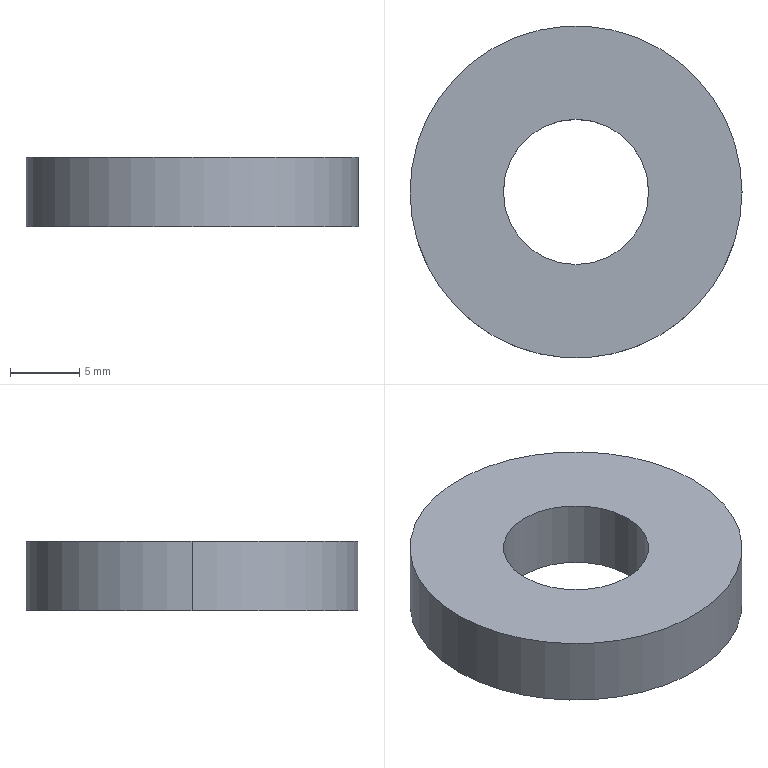Part | SolidWorks | features Extrusion 1 | 1 solid | 6 faces | box 24 x 24 x 5 mm | volume 1829 mm3 | cylinder 4 | plane 2 | commonest cylinder face diameters 10.5 x2 24 x2
STEP:
#1=CARTESIAN_POINT('',(-5.25,0.,5.));
#2=VERTEX_POINT('',#1);
#3=CARTESIAN_POINT('',(5.25,0.,5.));
#4=VERTEX_POINT('',#3);
#5=CARTESIAN_POINT('',(0.,0.,5.));
#6=DIRECTION('',(0.,0.,1.));
#7=DIRECTION('',(1.,0.,0.));
#8=AXIS2_PLACEMENT_3D('',#5,#6,#7);
#9=CIRCLE('',#8,5.25);
#10=EDGE_CURVE('',#2,#4,#9,.T.);
#11=ORIENTED_EDGE('',*,*,#10,.T.);
#12=CARTESIAN_POINT('',(5.25,0.,0.));
#13=VERTEX_POINT('',#12);
#14=CARTESIAN_POINT('',(5.25,0.,5.));
#15=DIRECTION('',(0.,0.,-1.));
#16=VECTOR('',#15,1000.);
#17=LINE('',#14,#16);
#18=EDGE_CURVE('',#4,#13,#17,.T.);
#19=ORIENTED_EDGE('',*,*,#18,.T.);
#20=CARTESIAN_POINT('',(-5.25,0.,0.));
#21=VERTEX_POINT('',#20);
#22=CARTESIAN_POINT('',(0.,0.,0.));
#23=DIRECTION('',(0.,0.,1.));
#24=DIRECTION('',(1.,0.,0.));
#25=AXIS2_PLACEMENT_3D('',#22,#23,#24);
#26=CIRCLE('',#25,5.25);
#27=EDGE_CURVE('',#21,#13,#26,.T.);
#28=ORIENTED_EDGE('',*,*,#27,.F.);
#29=CARTESIAN_POINT('',(-5.25,0.,5.));
#30=DIRECTION('',(0.,0.,-1.));
#31=VECTOR('',#30,1000.);
#32=LINE('',#29,#31);
#33=EDGE_CURVE('',#2,#21,#32,.T.);
#34=ORIENTED_EDGE('',*,*,#33,.F.);
#35=EDGE_LOOP('',(#11,#19,#28,#34));
#36=FACE_OUTER_BOUND('',#35,.T.);
#37=CARTESIAN_POINT('',(0.,0.,5.));
#38=DIRECTION('',(0.,0.,-1.));
#39=DIRECTION('',(-1.,0.,0.));
#40=AXIS2_PLACEMENT_3D('',#37,#38,#39);
#41=CYLINDRICAL_SURFACE('',#40,5.25);
#42=ADVANCED_FACE('',(#36),#41,.F.);
#43=CARTESIAN_POINT('',(12.,0.,5.));
#44=VERTEX_POINT('',#43);
#45=CARTESIAN_POINT('',(-12.,0.,5.));
#46=VERTEX_POINT('',#45);
#47=CARTESIAN_POINT('',(0.,0.,5.));
#48=DIRECTION('',(0.,0.,1.));
#49=DIRECTION('',(1.,0.,0.));
#50=AXIS2_PLACEMENT_3D('',#47,#48,#49);
#51=CIRCLE('',#50,12.);
#52=EDGE_CURVE('',#44,#46,#51,.T.);
#53=ORIENTED_EDGE('',*,*,#52,.F.);
#54=CARTESIAN_POINT('',(12.,0.,0.));
#55=VERTEX_POINT('',#54);
#56=CARTESIAN_POINT('',(12.,0.,5.));
#57=DIRECTION('',(0.,0.,-1.));
#58=VECTOR('',#57,1000.);
#59=LINE('',#56,#58);
#60=EDGE_CURVE('',#44,#55,#59,.T.);
#61=ORIENTED_EDGE('',*,*,#60,.T.);
#62=CARTESIAN_POINT('',(-12.,0.,0.));
#63=VERTEX_POINT('',#62);
#64=CARTESIAN_POINT('',(0.,0.,0.));
#65=DIRECTION('',(0.,0.,1.));
#66=DIRECTION('',(1.,0.,0.));
#67=AXIS2_PLACEMENT_3D('',#64,#65,#66);
#68=CIRCLE('',#67,12.);
#69=EDGE_CURVE('',#55,#63,#68,.T.);
#70=ORIENTED_EDGE('',*,*,#69,.T.);
#71=CARTESIAN_POINT('',(-12.,0.,5.));
#72=DIRECTION('',(0.,0.,-1.));
#73=VECTOR('',#72,1000.);
#74=LINE('',#71,#73);
#75=EDGE_CURVE('',#46,#63,#74,.T.);
#76=ORIENTED_EDGE('',*,*,#75,.F.);
#77=EDGE_LOOP('',(#53,#61,#70,#76));
#78=FACE_OUTER_BOUND('',#77,.T.);
#79=CARTESIAN_POINT('',(0.,0.,5.));
#80=DIRECTION('',(0.,0.,-1.));
#81=DIRECTION('',(-1.,0.,0.));
#82=AXIS2_PLACEMENT_3D('',#79,#80,#81);
#83=CYLINDRICAL_SURFACE('',#82,12.);
#84=ADVANCED_FACE('',(#78),#83,.T.);
#85=CARTESIAN_POINT('',(0.,0.,5.));
#86=DIRECTION('',(0.,0.,1.));
#87=DIRECTION('',(1.,0.,0.));
#88=AXIS2_PLACEMENT_3D('',#85,#86,#87);
#89=CIRCLE('',#88,12.);
#90=EDGE_CURVE('',#46,#44,#89,.T.);
#91=ORIENTED_EDGE('',*,*,#90,.T.);
#92=ORIENTED_EDGE('',*,*,#52,.T.);
#93=EDGE_LOOP('',(#91,#92));
#94=FACE_OUTER_BOUND('',#93,.T.);
#95=ORIENTED_EDGE('',*,*,#10,.F.);
#96=CARTESIAN_POINT('',(0.,0.,5.));
#97=DIRECTION('',(0.,0.,1.));
#98=DIRECTION('',(1.,0.,0.));
#99=AXIS2_PLACEMENT_3D('',#96,#97,#98);
#100=CIRCLE('',#99,5.25);
#101=EDGE_CURVE('',#4,#2,#100,.T.);
#102=ORIENTED_EDGE('',*,*,#101,.F.);
#103=EDGE_LOOP('',(#95,#102));
#104=FACE_BOUND('',#103,.T.);
#105=CARTESIAN_POINT('',(0.,0.,5.));
#106=DIRECTION('',(0.,0.,1.));
#107=DIRECTION('',(1.,0.,0.));
#108=AXIS2_PLACEMENT_3D('',#105,#106,#107);
#109=PLANE('',#108);
#110=ADVANCED_FACE('',(#94,#104),#109,.T.);
#111=CARTESIAN_POINT('',(0.,0.,0.));
#112=DIRECTION('',(0.,0.,1.));
#113=DIRECTION('',(1.,0.,0.));
#114=AXIS2_PLACEMENT_3D('',#111,#112,#113);
#115=CIRCLE('',#114,12.);
#116=EDGE_CURVE('',#63,#55,#115,.T.);
#117=ORIENTED_EDGE('',*,*,#116,.F.);
#118=ORIENTED_EDGE('',*,*,#69,.F.);
#119=EDGE_LOOP('',(#117,#118));
#120=FACE_OUTER_BOUND('',#119,.T.);
#121=ORIENTED_EDGE('',*,*,#27,.T.);
#122=CARTESIAN_POINT('',(0.,0.,0.));
#123=DIRECTION('',(0.,0.,1.));
#124=DIRECTION('',(1.,0.,0.));
#125=AXIS2_PLACEMENT_3D('',#122,#123,#124);
#126=CIRCLE('',#125,5.25);
#127=EDGE_CURVE('',#13,#21,#126,.T.);
#128=ORIENTED_EDGE('',*,*,#127,.T.);
#129=EDGE_LOOP('',(#121,#128));
#130=FACE_BOUND('',#129,.T.);
#131=CARTESIAN_POINT('',(0.,0.,0.));
#132=DIRECTION('',(0.,0.,1.));
#133=DIRECTION('',(1.,0.,0.));
#134=AXIS2_PLACEMENT_3D('',#131,#132,#133);
#135=PLANE('',#134);
#136=ADVANCED_FACE('',(#120,#130),#135,.F.);
#137=ORIENTED_EDGE('',*,*,#60,.F.);
#138=ORIENTED_EDGE('',*,*,#90,.F.);
#139=ORIENTED_EDGE('',*,*,#75,.T.);
#140=ORIENTED_EDGE('',*,*,#116,.T.);
#141=EDGE_LOOP('',(#137,#138,#139,#140));
#142=FACE_OUTER_BOUND('',#141,.T.);
#143=CARTESIAN_POINT('',(0.,0.,5.));
#144=DIRECTION('',(0.,0.,-1.));
#145=DIRECTION('',(-1.,0.,0.));
#146=AXIS2_PLACEMENT_3D('',#143,#144,#145);
#147=CYLINDRICAL_SURFACE('',#146,12.);
#148=ADVANCED_FACE('',(#142),#147,.T.);
#149=ORIENTED_EDGE('',*,*,#18,.F.);
#150=ORIENTED_EDGE('',*,*,#101,.T.);
#151=ORIENTED_EDGE('',*,*,#33,.T.);
#152=ORIENTED_EDGE('',*,*,#127,.F.);
#153=EDGE_LOOP('',(#149,#150,#151,#152));
#154=FACE_OUTER_BOUND('',#153,.T.);
#155=CARTESIAN_POINT('',(0.,0.,5.));
#156=DIRECTION('',(0.,0.,-1.));
#157=DIRECTION('',(-1.,0.,0.));
#158=AXIS2_PLACEMENT_3D('',#155,#156,#157);
#159=CYLINDRICAL_SURFACE('',#158,5.25);
#160=ADVANCED_FACE('',(#154),#159,.F.);
#161=CLOSED_SHELL('',(#42,#84,#110,#136,#148,#160));
#162=MANIFOLD_SOLID_BREP('',#161);
#163=CARTESIAN_POINT('',(0.,0.,0.));
#164=DIRECTION('',(0.,0.,1.));
#165=DIRECTION('',(1.,0.,0.));
#166=AXIS2_PLACEMENT_3D('',#163,#164,#165);
#167=(LENGTH_UNIT()NAMED_UNIT(*)SI_UNIT(.MILLI.,.METRE.));
#168=UNCERTAINTY_MEASURE_WITH_UNIT(LENGTH_MEASURE(0.00001),#167,'','');
#169=(NAMED_UNIT(*)PLANE_ANGLE_UNIT()SI_UNIT($,.RADIAN.));
#170=(NAMED_UNIT(*)SI_UNIT($,.STERADIAN.)SOLID_ANGLE_UNIT());
#171=(GEOMETRIC_REPRESENTATION_CONTEXT(3)GLOBAL_UNCERTAINTY_ASSIGNED_CONTEXT((#168))GLOBAL_UNIT_ASSIGNED_CONTEXT((#167,#169,#170))REPRESENTATION_CONTEXT('',''));
#172=ADVANCED_BREP_SHAPE_REPRESENTATION('',(#162,#166),#171);